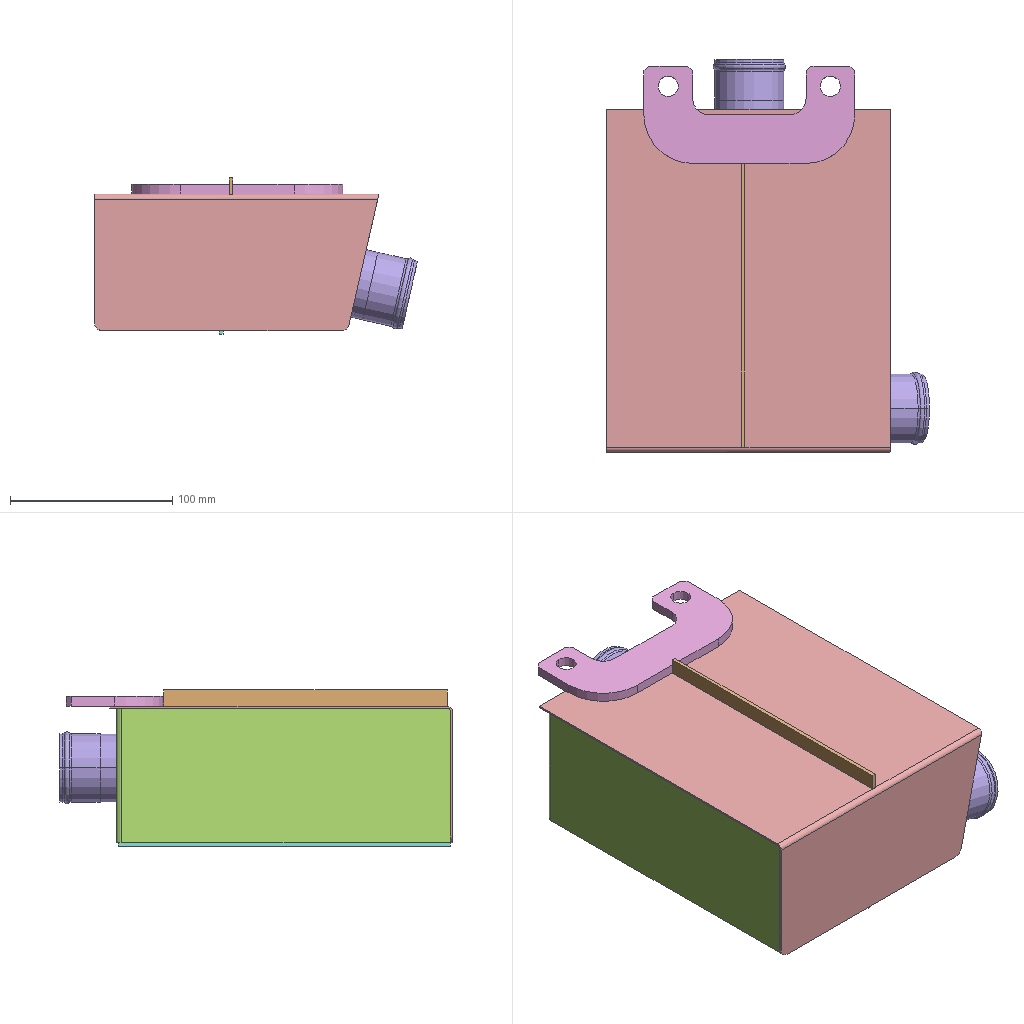Assembly | SolidWorks | 7 different items | 8 placed | box 199 x 242 x 96 mm
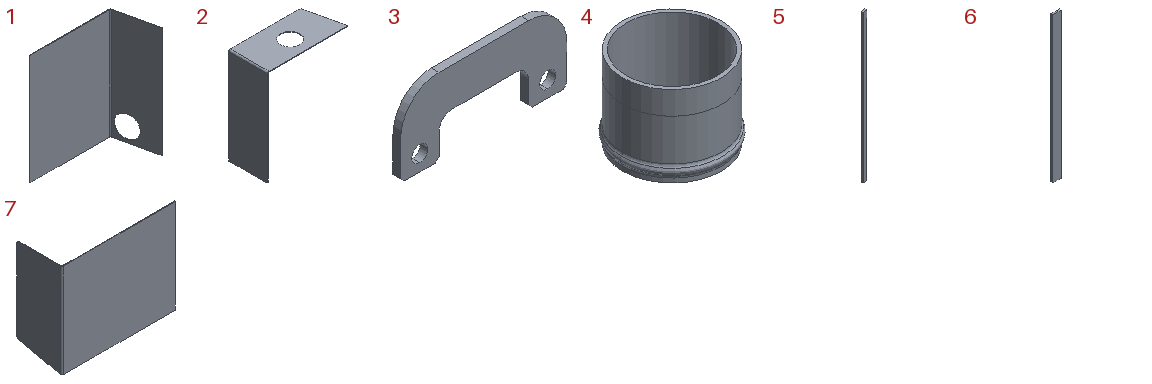Parts list (item | quantity | size | volume | features):
1 | x1 | 168 x 80.263 x 204.8 mm | 55034 mm3 | features Fillet 1, FlatPattern 1, ICE 1, SMBaseFlange 1, SheetMetal 1
2 | x1 | 171.49 x 83 x 206 mm | 34881 mm3 | features Fillet 2, FlatPattern 1, ICE 1, SMBaseFlange 1, SheetMetal 1
3 | x1 | 130 x 6 x 60 mm | 30559 mm3 | features FlatPattern 1, SMBaseFlange 1, SheetMetal 1
4 | x2 | 44.7 x 44.7 x 35 mm | 7344 mm3 | features ICE 1, RevolutionThin 1
5 | x1 | 5 x 2.3 x 204.8 mm | 2355 mm3 | features FlatPattern 1, SMBaseFlange 1, SheetMetal 1
6 | x1 | 10 x 2.3 x 175 mm | 4025 mm3 | features FlatPattern 1, SMBaseFlange 1, SheetMetal 1
7 | x1 | 211.2 x 84.2 x 175 mm | 60591 mm3 | features Fillet 1, FlatPattern 1, ICE 1, SMBaseFlange 1, SheetMetal 1
Mates (type | each side: item.copy, entity, surface, feature):
Coincident | 7.1 face plane Base-Flange1 | 1.1 face plane Base-Flange1
Coincident | 7.1 face plane Base-Flange1 | 2.1 face plane Base-Flange1 | 2 times
DistanceDim | 2.1 face plane Base-Flange1 | 7.1 face plane Base-Flange1
Coincident | 1.1 face plane Base-Flange1 | 2.1 face plane Base-Flange1
DistanceDim | 1.1 face plane Base-Flange1 | 7.1 face plane Base-Flange1
Coincident | 7.1 face plane Base-Flange1 | 3.1 face plane Base-Flange1
DistanceDim | 3.1 face plane Base-Flange1 | 7.1 face plane Base-Flange1 | 2 times
Coincident | 1.1 face plane Base-Flange1 | 5.1 face plane Base-Flange1
Coincident | 7.1 face plane Base-Flange1 | 5.1 face plane Base-Flange1
DistanceDim | 2.1 face plane Base-Flange1 | 5.1 face plane Base-Flange1
Coincident | 7.1 face plane Base-Flange1 | 6.1 face plane Base-Flange1
DistanceDim | 6.1 face plane Base-Flange1 | 7.1 face plane Base-Flange1
Coincident | 3.1 face plane Base-Flange1 | 6.1 face plane Base-Flange1
Coincident | 1.1 face plane Base-Flange1 | 4.1 face plane Revolve-Thin1
Concentric | 1.1 face cylinder Cut-Extrude1 | 4.1 face cylinder Revolve-Thin1
Parallel | 4.1 plane | assembly plane
Coincident | 2.1 face plane Base-Flange1 | 4.2 face plane Revolve-Thin1
Concentric | 2.1 face cylinder Cut-Extrude1 | 4.2 face cylinder Revolve-Thin1
Parallel | 4.2 plane | assembly plane